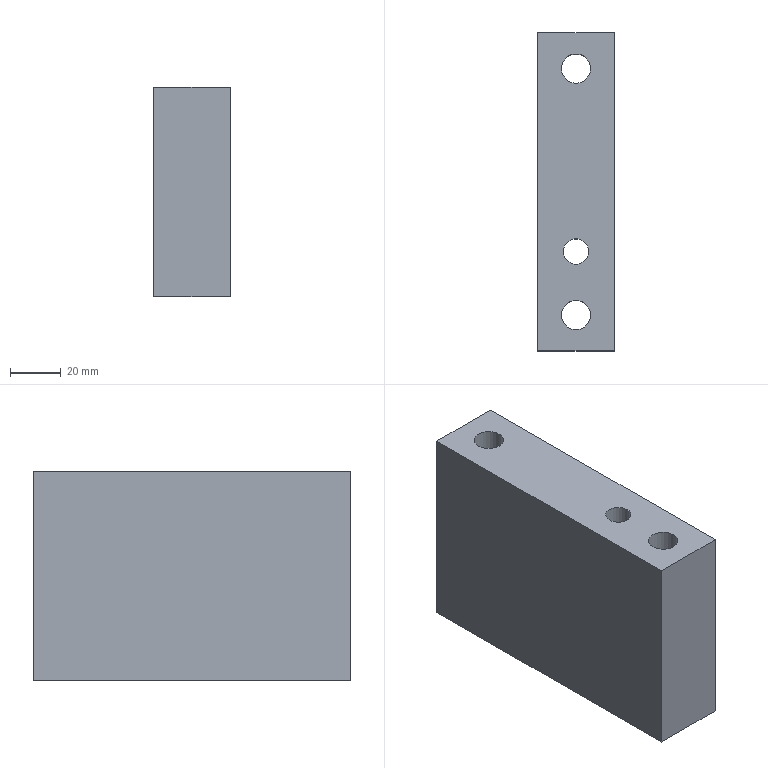Part | STEP file | lll_id3326_x_t | 1 solid | 32 faces | box 30 x 125 x 82.5 mm | volume 256192 mm3 | cylinder 20 | plane 12 | commonest cylinder face diameters 11.509 x2 18.007 x2 10 x1 13 x1 19.107 x1 19.147 x1
STEP:
#1=CARTESIAN_POINT('',(2265.,173.338,0.));
#2=VERTEX_POINT('',#1);
#3=CARTESIAN_POINT('',(2260.552,168.136,0.));
#4=VERTEX_POINT('',#3);
#5=CARTESIAN_POINT('',(2254.318,177.969,0.));
#6=DIRECTION('',(0.,0.,-1.));
#7=DIRECTION('',(-1.,0.,0.));
#8=AXIS2_PLACEMENT_3D('',#5,#6,#7);
#9=CIRCLE('',#8,11.642);
#10=EDGE_CURVE('',#2,#4,#9,.T.);
#11=ORIENTED_EDGE('',*,*,#10,.T.);
#12=CARTESIAN_POINT('',(2259.805,167.674,0.));
#13=VERTEX_POINT('',#12);
#14=CARTESIAN_POINT('',(2235.43,207.856,0.));
#15=DIRECTION('',(0.,0.,-1.));
#16=DIRECTION('',(-1.,0.,0.));
#17=AXIS2_PLACEMENT_3D('',#14,#15,#16);
#18=CIRCLE('',#17,46.998);
#19=EDGE_CURVE('',#4,#13,#18,.T.);
#20=ORIENTED_EDGE('',*,*,#19,.T.);
#21=CARTESIAN_POINT('',(2245.955,159.852,0.));
#22=VERTEX_POINT('',#21);
#23=CARTESIAN_POINT('',(2124.125,91.053,0.));
#24=DIRECTION('',(-0.8708,-0.4917,0.));
#25=VECTOR('',#24,1.);
#26=LINE('',#23,#25);
#27=EDGE_CURVE('',#13,#22,#26,.T.);
#28=ORIENTED_EDGE('',*,*,#27,.T.);
#29=CARTESIAN_POINT('',(2245.15,159.31,0.));
#30=VERTEX_POINT('',#29);
#31=CARTESIAN_POINT('',(2264.255,131.809,0.));
#32=DIRECTION('',(0.,0.,1.));
#33=DIRECTION('',(-1.,0.,0.));
#34=AXIS2_PLACEMENT_3D('',#31,#32,#33);
#35=CIRCLE('',#34,33.486);
#36=EDGE_CURVE('',#22,#30,#35,.T.);
#37=ORIENTED_EDGE('',*,*,#36,.T.);
#38=CARTESIAN_POINT('',(2244.347,158.71,0.));
#39=VERTEX_POINT('',#38);
#40=CARTESIAN_POINT('',(2252.954,148.02,0.));
#41=DIRECTION('',(0.,0.,1.));
#42=DIRECTION('',(-1.,0.,0.));
#43=AXIS2_PLACEMENT_3D('',#40,#41,#42);
#44=CIRCLE('',#43,13.725);
#45=EDGE_CURVE('',#30,#39,#44,.T.);
#46=ORIENTED_EDGE('',*,*,#45,.T.);
#47=CARTESIAN_POINT('',(2242.982,157.369,0.));
#48=VERTEX_POINT('',#47);
#49=CARTESIAN_POINT('',(2250.34,151.245,0.));
#50=DIRECTION('',(0.,0.,1.));
#51=DIRECTION('',(-1.,0.,0.));
#52=AXIS2_PLACEMENT_3D('',#49,#50,#51);
#53=CIRCLE('',#52,9.573);
#54=EDGE_CURVE('',#39,#48,#53,.T.);
#55=ORIENTED_EDGE('',*,*,#54,.T.);
#56=CARTESIAN_POINT('',(2240.441,151.267,0.));
#57=VERTEX_POINT('',#56);
#58=CARTESIAN_POINT('',(2251.719,150.151,0.));
#59=DIRECTION('',(0.,0.,1.));
#60=DIRECTION('',(-1.,0.,0.));
#61=AXIS2_PLACEMENT_3D('',#58,#59,#60);
#62=CIRCLE('',#61,11.334);
#63=EDGE_CURVE('',#48,#57,#62,.T.);
#64=ORIENTED_EDGE('',*,*,#63,.T.);
#65=CARTESIAN_POINT('',(2244.304,142.034,0.));
#66=VERTEX_POINT('',#65);
#67=CARTESIAN_POINT('',(2251.482,150.461,0.));
#68=DIRECTION('',(0.,0.,-1.));
#69=DIRECTION('',(-1.,0.,0.));
#70=AXIS2_PLACEMENT_3D('',#67,#68,#69);
#71=CIRCLE('',#70,11.07);
#72=EDGE_CURVE('',#66,#57,#71,.T.);
#73=ORIENTED_EDGE('',*,*,#72,.F.);
#74=CARTESIAN_POINT('',(2245.194,141.368,0.));
#75=VERTEX_POINT('',#74);
#76=CARTESIAN_POINT('',(2251.305,150.47,0.));
#77=DIRECTION('',(0.,0.,-1.));
#78=DIRECTION('',(-1.,0.,0.));
#79=AXIS2_PLACEMENT_3D('',#76,#77,#78);
#80=CIRCLE('',#79,10.964);
#81=EDGE_CURVE('',#75,#66,#80,.T.);
#82=ORIENTED_EDGE('',*,*,#81,.F.);
#83=CARTESIAN_POINT('',(2246.008,140.845,0.));
#84=VERTEX_POINT('',#83);
#85=CARTESIAN_POINT('',(2258.447,161.108,0.));
#86=DIRECTION('',(0.,0.,-1.));
#87=DIRECTION('',(-1.,0.,0.));
#88=AXIS2_PLACEMENT_3D('',#85,#86,#87);
#89=CIRCLE('',#88,23.776);
#90=EDGE_CURVE('',#84,#75,#89,.T.);
#91=ORIENTED_EDGE('',*,*,#90,.F.);
#92=CARTESIAN_POINT('',(2259.795,133.095,0.));
#93=VERTEX_POINT('',#92);
#94=CARTESIAN_POINT('',(2403.433,52.349,0.));
#95=DIRECTION('',(-0.8717,0.49,0.));
#96=VECTOR('',#95,1.);
#97=LINE('',#94,#96);
#98=EDGE_CURVE('',#93,#84,#97,.T.);
#99=ORIENTED_EDGE('',*,*,#98,.F.);
#100=CARTESIAN_POINT('',(2260.503,132.626,0.));
#101=VERTEX_POINT('',#100);
#102=CARTESIAN_POINT('',(2230.701,88.407,0.));
#103=DIRECTION('',(0.,0.,1.));
#104=DIRECTION('',(-1.,0.,0.));
#105=AXIS2_PLACEMENT_3D('',#102,#103,#104);
#106=CIRCLE('',#105,53.324);
#107=EDGE_CURVE('',#101,#93,#106,.T.);
#108=ORIENTED_EDGE('',*,*,#107,.F.);
#109=CARTESIAN_POINT('',(2261.24,132.116,0.));
#110=VERTEX_POINT('',#109);
#111=CARTESIAN_POINT('',(2244.874,109.242,0.));
#112=DIRECTION('',(0.,0.,1.));
#113=DIRECTION('',(-1.,0.,0.));
#114=AXIS2_PLACEMENT_3D('',#111,#112,#113);
#115=CIRCLE('',#114,28.126);
#116=EDGE_CURVE('',#110,#101,#115,.T.);
#117=ORIENTED_EDGE('',*,*,#116,.F.);
#118=CARTESIAN_POINT('',(2261.899,131.617,0.));
#119=VERTEX_POINT('',#118);
#120=CARTESIAN_POINT('',(2252.238,119.534,0.));
#121=DIRECTION('',(0.,0.,1.));
#122=DIRECTION('',(-1.,0.,0.));
#123=AXIS2_PLACEMENT_3D('',#120,#121,#122);
#124=CIRCLE('',#123,15.471);
#125=EDGE_CURVE('',#119,#110,#124,.T.);
#126=ORIENTED_EDGE('',*,*,#125,.F.);
#127=CARTESIAN_POINT('',(2262.589,131.012,0.));
#128=VERTEX_POINT('',#127);
#129=CARTESIAN_POINT('',(2255.947,124.145,0.));
#130=DIRECTION('',(0.,0.,1.));
#131=DIRECTION('',(-1.,0.,0.));
#132=AXIS2_PLACEMENT_3D('',#129,#130,#131);
#133=CIRCLE('',#132,9.553);
#134=EDGE_CURVE('',#128,#119,#133,.T.);
#135=ORIENTED_EDGE('',*,*,#134,.F.);
#136=CARTESIAN_POINT('',(2265.,127.474,0.));
#137=VERTEX_POINT('',#136);
#138=CARTESIAN_POINT('',(2254.53,122.929,0.));
#139=DIRECTION('',(0.,0.,1.));
#140=DIRECTION('',(-1.,0.,0.));
#141=AXIS2_PLACEMENT_3D('',#138,#139,#140);
#142=CIRCLE('',#141,11.414);
#143=EDGE_CURVE('',#137,#128,#142,.T.);
#144=ORIENTED_EDGE('',*,*,#143,.F.);
#145=CARTESIAN_POINT('',(2265.,75.,0.));
#146=VERTEX_POINT('',#145);
#147=CARTESIAN_POINT('',(2265.,4.,0.));
#148=DIRECTION('',(0.,1.,0.));
#149=VECTOR('',#148,1.);
#150=LINE('',#147,#149);
#151=EDGE_CURVE('',#146,#137,#150,.T.);
#152=ORIENTED_EDGE('',*,*,#151,.F.);
#153=CARTESIAN_POINT('',(2235.,75.,0.));
#154=VERTEX_POINT('',#153);
#155=CARTESIAN_POINT('',(2275.,75.,0.));
#156=DIRECTION('',(1.,0.,0.));
#157=VECTOR('',#156,1.);
#158=LINE('',#155,#157);
#159=EDGE_CURVE('',#154,#146,#158,.T.);
#160=ORIENTED_EDGE('',*,*,#159,.F.);
#161=CARTESIAN_POINT('',(2235.,200.,0.));
#162=VERTEX_POINT('',#161);
#163=CARTESIAN_POINT('',(2235.,-176.117,0.));
#164=DIRECTION('',(0.,1.,0.));
#165=VECTOR('',#164,1.);
#166=LINE('',#163,#165);
#167=EDGE_CURVE('',#154,#162,#166,.T.);
#168=ORIENTED_EDGE('',*,*,#167,.T.);
#169=CARTESIAN_POINT('',(2265.,200.,0.));
#170=VERTEX_POINT('',#169);
#171=CARTESIAN_POINT('',(2250.,200.,0.));
#172=DIRECTION('',(-1.,0.,0.));
#173=VECTOR('',#172,1.);
#174=LINE('',#171,#173);
#175=EDGE_CURVE('',#170,#162,#174,.T.);
#176=ORIENTED_EDGE('',*,*,#175,.F.);
#177=CARTESIAN_POINT('',(2265.,4.,0.));
#178=DIRECTION('',(0.,1.,0.));
#179=VECTOR('',#178,1.);
#180=LINE('',#177,#179);
#181=EDGE_CURVE('',#2,#170,#180,.T.);
#182=ORIENTED_EDGE('',*,*,#181,.F.);
#183=EDGE_LOOP('',(#11,#20,#28,#37,#46,#55,#64,#73,#82,#91,#99,#108,#117,#126,#135,#144,#152,#160,#168,#176,#182));
#184=FACE_BOUND('',#183,.T.);
#185=CARTESIAN_POINT('',(2240.997,89.,0.));
#186=VERTEX_POINT('',#185);
#187=CARTESIAN_POINT('',(2250.,89.,0.));
#188=DIRECTION('',(0.,0.,-1.));
#189=DIRECTION('',(-1.,0.,0.));
#190=AXIS2_PLACEMENT_3D('',#187,#188,#189);
#191=CIRCLE('',#190,9.004);
#192=EDGE_CURVE('',#186,#186,#191,.T.);
#193=ORIENTED_EDGE('',*,*,#192,.F.);
#194=EDGE_LOOP('',(#193));
#195=FACE_BOUND('',#194,.T.);
#196=CARTESIAN_POINT('',(2240.997,186.,0.));
#197=VERTEX_POINT('',#196);
#198=CARTESIAN_POINT('',(2250.,186.,0.));
#199=DIRECTION('',(0.,0.,-1.));
#200=DIRECTION('',(-1.,0.,0.));
#201=AXIS2_PLACEMENT_3D('',#198,#199,#200);
#202=CIRCLE('',#201,9.004);
#203=EDGE_CURVE('',#197,#197,#202,.T.);
#204=ORIENTED_EDGE('',*,*,#203,.F.);
#205=EDGE_LOOP('',(#204));
#206=FACE_BOUND('',#205,.T.);
#207=CARTESIAN_POINT('',(2256.5,114.,0.));
#208=VERTEX_POINT('',#207);
#209=CARTESIAN_POINT('',(2250.,114.,0.));
#210=DIRECTION('',(0.,0.,1.));
#211=DIRECTION('',(1.,0.,0.));
#212=AXIS2_PLACEMENT_3D('',#209,#210,#211);
#213=CIRCLE('',#212,6.5);
#214=EDGE_CURVE('',#208,#208,#213,.T.);
#215=ORIENTED_EDGE('',*,*,#214,.T.);
#216=EDGE_LOOP('',(#215));
#217=FACE_BOUND('',#216,.T.);
#218=CARTESIAN_POINT('',(2275.,-176.117,0.));
#219=DIRECTION('',(0.,0.,-1.));
#220=DIRECTION('',(-1.,0.,0.));
#221=AXIS2_PLACEMENT_3D('',#218,#219,#220);
#222=PLANE('',#221);
#223=ADVANCED_FACE('',(#184,#195,#206,#217),#222,.T.);
#224=CARTESIAN_POINT('',(2259.003,186.,52.5));
#225=VERTEX_POINT('',#224);
#226=CARTESIAN_POINT('',(2250.,186.,52.5));
#227=DIRECTION('',(0.,0.,-1.));
#228=DIRECTION('',(1.,0.,0.));
#229=AXIS2_PLACEMENT_3D('',#226,#227,#228);
#230=CIRCLE('',#229,9.004);
#231=EDGE_CURVE('',#225,#225,#230,.T.);
#232=ORIENTED_EDGE('',*,*,#231,.F.);
#233=EDGE_LOOP('',(#232));
#234=FACE_BOUND('',#233,.T.);
#235=ORIENTED_EDGE('',*,*,#203,.T.);
#236=EDGE_LOOP('',(#235));
#237=FACE_BOUND('',#236,.T.);
#238=CARTESIAN_POINT('',(2250.,186.,2.5));
#239=DIRECTION('',(0.,0.,1.));
#240=DIRECTION('',(1.,0.,0.));
#241=AXIS2_PLACEMENT_3D('',#238,#239,#240);
#242=CYLINDRICAL_SURFACE('',#241,9.004);
#243=ADVANCED_FACE('',(#234,#237),#242,.F.);
#244=CARTESIAN_POINT('',(2259.003,89.,52.5));
#245=VERTEX_POINT('',#244);
#246=CARTESIAN_POINT('',(2250.,89.,52.5));
#247=DIRECTION('',(0.,0.,-1.));
#248=DIRECTION('',(1.,0.,0.));
#249=AXIS2_PLACEMENT_3D('',#246,#247,#248);
#250=CIRCLE('',#249,9.004);
#251=EDGE_CURVE('',#245,#245,#250,.T.);
#252=ORIENTED_EDGE('',*,*,#251,.F.);
#253=EDGE_LOOP('',(#252));
#254=FACE_BOUND('',#253,.T.);
#255=ORIENTED_EDGE('',*,*,#192,.T.);
#256=EDGE_LOOP('',(#255));
#257=FACE_BOUND('',#256,.T.);
#258=CARTESIAN_POINT('',(2250.,89.,2.5));
#259=DIRECTION('',(0.,0.,1.));
#260=DIRECTION('',(1.,0.,0.));
#261=AXIS2_PLACEMENT_3D('',#258,#259,#260);
#262=CYLINDRICAL_SURFACE('',#261,9.004);
#263=ADVANCED_FACE('',(#254,#257),#262,.F.);
#264=CARTESIAN_POINT('',(2265.,127.474,17.));
#265=VERTEX_POINT('',#264);
#266=CARTESIAN_POINT('',(2265.,127.474,2.5));
#267=DIRECTION('',(0.,0.,1.));
#268=VECTOR('',#267,1.);
#269=LINE('',#266,#268);
#270=EDGE_CURVE('',#137,#265,#269,.T.);
#271=ORIENTED_EDGE('',*,*,#270,.T.);
#272=CARTESIAN_POINT('',(2265.,173.338,17.));
#273=VERTEX_POINT('',#272);
#274=CARTESIAN_POINT('',(2265.,4.,17.));
#275=DIRECTION('',(0.,1.,0.));
#276=VECTOR('',#275,1.);
#277=LINE('',#274,#276);
#278=EDGE_CURVE('',#265,#273,#277,.T.);
#279=ORIENTED_EDGE('',*,*,#278,.T.);
#280=CARTESIAN_POINT('',(2265.,173.338,5.5));
#281=DIRECTION('',(0.,0.,-1.));
#282=VECTOR('',#281,1.);
#283=LINE('',#280,#282);
#284=EDGE_CURVE('',#273,#2,#283,.T.);
#285=ORIENTED_EDGE('',*,*,#284,.T.);
#286=ORIENTED_EDGE('',*,*,#181,.T.);
#287=CARTESIAN_POINT('',(2265.,200.,82.5));
#288=VERTEX_POINT('',#287);
#289=CARTESIAN_POINT('',(2265.,200.,-652.5));
#290=DIRECTION('',(0.,0.,-1.));
#291=VECTOR('',#290,1.);
#292=LINE('',#289,#291);
#293=EDGE_CURVE('',#288,#170,#292,.T.);
#294=ORIENTED_EDGE('',*,*,#293,.F.);
#295=CARTESIAN_POINT('',(2265.,75.,82.5));
#296=VERTEX_POINT('',#295);
#297=CARTESIAN_POINT('',(2265.,4.,82.5));
#298=DIRECTION('',(0.,-1.,0.));
#299=VECTOR('',#298,1.);
#300=LINE('',#297,#299);
#301=EDGE_CURVE('',#288,#296,#300,.T.);
#302=ORIENTED_EDGE('',*,*,#301,.T.);
#303=CARTESIAN_POINT('',(2265.,75.,40.));
#304=DIRECTION('',(0.,0.,-1.));
#305=VECTOR('',#304,1.);
#306=LINE('',#303,#305);
#307=EDGE_CURVE('',#296,#146,#306,.T.);
#308=ORIENTED_EDGE('',*,*,#307,.T.);
#309=ORIENTED_EDGE('',*,*,#151,.T.);
#310=EDGE_LOOP('',(#271,#279,#285,#286,#294,#302,#308,#309));
#311=FACE_OUTER_BOUND('',#310,.T.);
#312=CARTESIAN_POINT('',(2265.,4.,-652.5));
#313=DIRECTION('',(-1.,0.,0.));
#314=DIRECTION('',(0.,0.,1.));
#315=AXIS2_PLACEMENT_3D('',#312,#313,#314);
#316=PLANE('',#315);
#317=ADVANCED_FACE('',(#311),#316,.F.);
#318=CARTESIAN_POINT('',(2255.755,186.,82.5));
#319=VERTEX_POINT('',#318);
#320=CARTESIAN_POINT('',(2250.,186.,82.5));
#321=DIRECTION('',(0.,0.,-1.));
#322=DIRECTION('',(1.,0.,0.));
#323=AXIS2_PLACEMENT_3D('',#320,#321,#322);
#324=CIRCLE('',#323,5.755);
#325=EDGE_CURVE('',#319,#319,#324,.T.);
#326=ORIENTED_EDGE('',*,*,#325,.T.);
#327=EDGE_LOOP('',(#326));
#328=FACE_BOUND('',#327,.T.);
#329=CARTESIAN_POINT('',(2255.755,89.,82.5));
#330=VERTEX_POINT('',#329);
#331=CARTESIAN_POINT('',(2250.,89.,82.5));
#332=DIRECTION('',(0.,0.,-1.));
#333=DIRECTION('',(1.,0.,0.));
#334=AXIS2_PLACEMENT_3D('',#331,#332,#333);
#335=CIRCLE('',#334,5.755);
#336=EDGE_CURVE('',#330,#330,#335,.T.);
#337=ORIENTED_EDGE('',*,*,#336,.T.);
#338=EDGE_LOOP('',(#337));
#339=FACE_BOUND('',#338,.T.);
#340=CARTESIAN_POINT('',(2255.,114.,82.5));
#341=VERTEX_POINT('',#340);
#342=CARTESIAN_POINT('',(2250.,114.,82.5));
#343=DIRECTION('',(0.,0.,-1.));
#344=DIRECTION('',(1.,0.,0.));
#345=AXIS2_PLACEMENT_3D('',#342,#343,#344);
#346=CIRCLE('',#345,5.);
#347=EDGE_CURVE('',#341,#341,#346,.T.);
#348=ORIENTED_EDGE('',*,*,#347,.T.);
#349=EDGE_LOOP('',(#348));
#350=FACE_BOUND('',#349,.T.);
#351=CARTESIAN_POINT('',(2235.,200.,82.5));
#352=VERTEX_POINT('',#351);
#353=CARTESIAN_POINT('',(2275.,200.,82.5));
#354=DIRECTION('',(-1.,0.,0.));
#355=VECTOR('',#354,1.);
#356=LINE('',#353,#355);
#357=EDGE_CURVE('',#288,#352,#356,.T.);
#358=ORIENTED_EDGE('',*,*,#357,.T.);
#359=CARTESIAN_POINT('',(2235.,75.,82.5));
#360=VERTEX_POINT('',#359);
#361=CARTESIAN_POINT('',(2235.,4.,82.5));
#362=DIRECTION('',(0.,-1.,0.));
#363=VECTOR('',#362,1.);
#364=LINE('',#361,#363);
#365=EDGE_CURVE('',#352,#360,#364,.T.);
#366=ORIENTED_EDGE('',*,*,#365,.T.);
#367=CARTESIAN_POINT('',(2275.,75.,82.5));
#368=DIRECTION('',(1.,0.,0.));
#369=VECTOR('',#368,1.);
#370=LINE('',#367,#369);
#371=EDGE_CURVE('',#360,#296,#370,.T.);
#372=ORIENTED_EDGE('',*,*,#371,.T.);
#373=ORIENTED_EDGE('',*,*,#301,.F.);
#374=EDGE_LOOP('',(#358,#366,#372,#373));
#375=FACE_BOUND('',#374,.T.);
#376=CARTESIAN_POINT('',(2275.,236.117,82.5));
#377=DIRECTION('',(0.,0.,1.));
#378=DIRECTION('',(1.,0.,0.));
#379=AXIS2_PLACEMENT_3D('',#376,#377,#378);
#380=PLANE('',#379);
#381=ADVANCED_FACE('',(#328,#339,#350,#375),#380,.T.);
#382=CARTESIAN_POINT('',(2235.,200.,40.));
#383=DIRECTION('',(0.,0.,1.));
#384=VECTOR('',#383,1.);
#385=LINE('',#382,#384);
#386=EDGE_CURVE('',#162,#352,#385,.T.);
#387=ORIENTED_EDGE('',*,*,#386,.F.);
#388=ORIENTED_EDGE('',*,*,#167,.F.);
#389=CARTESIAN_POINT('',(2235.,75.,-652.5));
#390=DIRECTION('',(0.,0.,1.));
#391=VECTOR('',#390,1.);
#392=LINE('',#389,#391);
#393=EDGE_CURVE('',#154,#360,#392,.T.);
#394=ORIENTED_EDGE('',*,*,#393,.T.);
#395=ORIENTED_EDGE('',*,*,#365,.F.);
#396=EDGE_LOOP('',(#387,#388,#394,#395));
#397=FACE_OUTER_BOUND('',#396,.T.);
#398=CARTESIAN_POINT('',(2235.,4.,-652.5));
#399=DIRECTION('',(-1.,0.,0.));
#400=DIRECTION('',(0.,0.,1.));
#401=AXIS2_PLACEMENT_3D('',#398,#399,#400);
#402=PLANE('',#401);
#403=ADVANCED_FACE('',(#397),#402,.T.);
#404=ORIENTED_EDGE('',*,*,#159,.T.);
#405=ORIENTED_EDGE('',*,*,#307,.F.);
#406=ORIENTED_EDGE('',*,*,#371,.F.);
#407=ORIENTED_EDGE('',*,*,#393,.F.);
#408=EDGE_LOOP('',(#404,#405,#406,#407));
#409=FACE_OUTER_BOUND('',#408,.T.);
#410=CARTESIAN_POINT('',(2536.,75.,40.));
#411=DIRECTION('',(0.,1.,0.));
#412=DIRECTION('',(0.,0.,-1.));
#413=AXIS2_PLACEMENT_3D('',#410,#411,#412);
#414=PLANE('',#413);
#415=ADVANCED_FACE('',(#409),#414,.F.);
#416=ORIENTED_EDGE('',*,*,#357,.F.);
#417=ORIENTED_EDGE('',*,*,#293,.T.);
#418=ORIENTED_EDGE('',*,*,#175,.T.);
#419=ORIENTED_EDGE('',*,*,#386,.T.);
#420=EDGE_LOOP('',(#416,#417,#418,#419));
#421=FACE_OUTER_BOUND('',#420,.T.);
#422=CARTESIAN_POINT('',(2250.,200.,40.));
#423=DIRECTION('',(0.,-1.,0.));
#424=DIRECTION('',(0.,0.,1.));
#425=AXIS2_PLACEMENT_3D('',#422,#423,#424);
#426=PLANE('',#425);
#427=ADVANCED_FACE('',(#421),#426,.F.);
#428=ORIENTED_EDGE('',*,*,#270,.F.);
#429=ORIENTED_EDGE('',*,*,#143,.T.);
#430=CARTESIAN_POINT('',(2262.589,131.012,17.));
#431=VERTEX_POINT('',#430);
#432=CARTESIAN_POINT('',(2262.589,131.012,5.5));
#433=DIRECTION('',(0.,0.,-1.));
#434=VECTOR('',#433,1.);
#435=LINE('',#432,#434);
#436=EDGE_CURVE('',#431,#128,#435,.T.);
#437=ORIENTED_EDGE('',*,*,#436,.F.);
#438=CARTESIAN_POINT('',(2254.53,122.929,17.));
#439=DIRECTION('',(0.,0.,-1.));
#440=DIRECTION('',(-1.,0.,0.));
#441=AXIS2_PLACEMENT_3D('',#438,#439,#440);
#442=CIRCLE('',#441,11.414);
#443=EDGE_CURVE('',#431,#265,#442,.T.);
#444=ORIENTED_EDGE('',*,*,#443,.T.);
#445=EDGE_LOOP('',(#428,#429,#437,#444));
#446=FACE_OUTER_BOUND('',#445,.T.);
#447=CARTESIAN_POINT('',(2254.53,122.929,2.5));
#448=DIRECTION('',(0.,0.,-1.));
#449=DIRECTION('',(-1.,0.,0.));
#450=AXIS2_PLACEMENT_3D('',#447,#448,#449);
#451=CYLINDRICAL_SURFACE('',#450,11.414);
#452=ADVANCED_FACE('',(#446),#451,.T.);
#453=ORIENTED_EDGE('',*,*,#284,.F.);
#454=CARTESIAN_POINT('',(2260.552,168.136,17.));
#455=VERTEX_POINT('',#454);
#456=CARTESIAN_POINT('',(2254.318,177.969,17.));
#457=DIRECTION('',(0.,0.,1.));
#458=DIRECTION('',(-1.,0.,0.));
#459=AXIS2_PLACEMENT_3D('',#456,#457,#458);
#460=CIRCLE('',#459,11.642);
#461=EDGE_CURVE('',#455,#273,#460,.T.);
#462=ORIENTED_EDGE('',*,*,#461,.F.);
#463=CARTESIAN_POINT('',(2260.552,168.136,2.5));
#464=DIRECTION('',(0.,0.,-1.));
#465=VECTOR('',#464,1.);
#466=LINE('',#463,#465);
#467=EDGE_CURVE('',#455,#4,#466,.T.);
#468=ORIENTED_EDGE('',*,*,#467,.T.);
#469=ORIENTED_EDGE('',*,*,#10,.F.);
#470=EDGE_LOOP('',(#453,#462,#468,#469));
#471=FACE_OUTER_BOUND('',#470,.T.);
#472=CARTESIAN_POINT('',(2254.318,177.969,2.5));
#473=DIRECTION('',(0.,0.,-1.));
#474=DIRECTION('',(-1.,0.,0.));
#475=AXIS2_PLACEMENT_3D('',#472,#473,#474);
#476=CYLINDRICAL_SURFACE('',#475,11.642);
#477=ADVANCED_FACE('',(#471),#476,.T.);
#478=ORIENTED_EDGE('',*,*,#278,.F.);
#479=ORIENTED_EDGE('',*,*,#443,.F.);
#480=CARTESIAN_POINT('',(2261.899,131.617,17.));
#481=VERTEX_POINT('',#480);
#482=CARTESIAN_POINT('',(2255.947,124.145,17.));
#483=DIRECTION('',(0.,0.,-1.));
#484=DIRECTION('',(-1.,0.,0.));
#485=AXIS2_PLACEMENT_3D('',#482,#483,#484);
#486=CIRCLE('',#485,9.553);
#487=EDGE_CURVE('',#481,#431,#486,.T.);
#488=ORIENTED_EDGE('',*,*,#487,.F.);
#489=CARTESIAN_POINT('',(2261.24,132.116,17.));
#490=VERTEX_POINT('',#489);
#491=CARTESIAN_POINT('',(2252.238,119.534,17.));
#492=DIRECTION('',(0.,0.,-1.));
#493=DIRECTION('',(-1.,0.,0.));
#494=AXIS2_PLACEMENT_3D('',#491,#492,#493);
#495=CIRCLE('',#494,15.471);
#496=EDGE_CURVE('',#490,#481,#495,.T.);
#497=ORIENTED_EDGE('',*,*,#496,.F.);
#498=CARTESIAN_POINT('',(2260.503,132.626,17.));
#499=VERTEX_POINT('',#498);
#500=CARTESIAN_POINT('',(2244.874,109.242,17.));
#501=DIRECTION('',(0.,0.,-1.));
#502=DIRECTION('',(-1.,0.,0.));
#503=AXIS2_PLACEMENT_3D('',#500,#501,#502);
#504=CIRCLE('',#503,28.126);
#505=EDGE_CURVE('',#499,#490,#504,.T.);
#506=ORIENTED_EDGE('',*,*,#505,.F.);
#507=CARTESIAN_POINT('',(2259.795,133.095,17.));
#508=VERTEX_POINT('',#507);
#509=CARTESIAN_POINT('',(2230.701,88.407,17.));
#510=DIRECTION('',(0.,0.,-1.));
#511=DIRECTION('',(-1.,0.,0.));
#512=AXIS2_PLACEMENT_3D('',#509,#510,#511);
#513=CIRCLE('',#512,53.324);
#514=EDGE_CURVE('',#508,#499,#513,.T.);
#515=ORIENTED_EDGE('',*,*,#514,.F.);
#516=CARTESIAN_POINT('',(2246.008,140.845,17.));
#517=VERTEX_POINT('',#516);
#518=CARTESIAN_POINT('',(2259.879,133.048,17.));
#519=DIRECTION('',(0.8717,-0.49,0.));
#520=VECTOR('',#519,1.);
#521=LINE('',#518,#520);
#522=EDGE_CURVE('',#517,#508,#521,.T.);
#523=ORIENTED_EDGE('',*,*,#522,.F.);
#524=CARTESIAN_POINT('',(2245.194,141.368,17.));
#525=VERTEX_POINT('',#524);
#526=CARTESIAN_POINT('',(2258.447,161.108,17.));
#527=DIRECTION('',(0.,0.,1.));
#528=DIRECTION('',(-1.,0.,0.));
#529=AXIS2_PLACEMENT_3D('',#526,#527,#528);
#530=CIRCLE('',#529,23.776);
#531=EDGE_CURVE('',#525,#517,#530,.T.);
#532=ORIENTED_EDGE('',*,*,#531,.F.);
#533=CARTESIAN_POINT('',(2244.304,142.034,17.));
#534=VERTEX_POINT('',#533);
#535=CARTESIAN_POINT('',(2251.305,150.47,17.));
#536=DIRECTION('',(0.,0.,1.));
#537=DIRECTION('',(-1.,0.,0.));
#538=AXIS2_PLACEMENT_3D('',#535,#536,#537);
#539=CIRCLE('',#538,10.964);
#540=EDGE_CURVE('',#534,#525,#539,.T.);
#541=ORIENTED_EDGE('',*,*,#540,.F.);
#542=CARTESIAN_POINT('',(2240.441,151.267,17.));
#543=VERTEX_POINT('',#542);
#544=CARTESIAN_POINT('',(2251.482,150.461,17.));
#545=DIRECTION('',(0.,0.,1.));
#546=DIRECTION('',(-1.,0.,0.));
#547=AXIS2_PLACEMENT_3D('',#544,#545,#546);
#548=CIRCLE('',#547,11.07);
#549=EDGE_CURVE('',#543,#534,#548,.T.);
#550=ORIENTED_EDGE('',*,*,#549,.F.);
#551=CARTESIAN_POINT('',(2242.982,157.369,17.));
#552=VERTEX_POINT('',#551);
#553=CARTESIAN_POINT('',(2251.719,150.151,17.));
#554=DIRECTION('',(0.,0.,-1.));
#555=DIRECTION('',(-1.,0.,0.));
#556=AXIS2_PLACEMENT_3D('',#553,#554,#555);
#557=CIRCLE('',#556,11.334);
#558=EDGE_CURVE('',#543,#552,#557,.T.);
#559=ORIENTED_EDGE('',*,*,#558,.T.);
#560=CARTESIAN_POINT('',(2244.347,158.71,17.));
#561=VERTEX_POINT('',#560);
#562=CARTESIAN_POINT('',(2250.34,151.245,17.));
#563=DIRECTION('',(0.,0.,-1.));
#564=DIRECTION('',(-1.,0.,0.));
#565=AXIS2_PLACEMENT_3D('',#562,#563,#564);
#566=CIRCLE('',#565,9.573);
#567=EDGE_CURVE('',#552,#561,#566,.T.);
#568=ORIENTED_EDGE('',*,*,#567,.T.);
#569=CARTESIAN_POINT('',(2245.15,159.31,17.));
#570=VERTEX_POINT('',#569);
#571=CARTESIAN_POINT('',(2252.954,148.02,17.));
#572=DIRECTION('',(0.,0.,-1.));
#573=DIRECTION('',(-1.,0.,0.));
#574=AXIS2_PLACEMENT_3D('',#571,#572,#573);
#575=CIRCLE('',#574,13.725);
#576=EDGE_CURVE('',#561,#570,#575,.T.);
#577=ORIENTED_EDGE('',*,*,#576,.T.);
#578=CARTESIAN_POINT('',(2245.955,159.852,17.));
#579=VERTEX_POINT('',#578);
#580=CARTESIAN_POINT('',(2264.255,131.809,17.));
#581=DIRECTION('',(0.,0.,-1.));
#582=DIRECTION('',(-1.,0.,0.));
#583=AXIS2_PLACEMENT_3D('',#580,#581,#582);
#584=CIRCLE('',#583,33.486);
#585=EDGE_CURVE('',#570,#579,#584,.T.);
#586=ORIENTED_EDGE('',*,*,#585,.T.);
#587=CARTESIAN_POINT('',(2259.805,167.674,17.));
#588=VERTEX_POINT('',#587);
#589=CARTESIAN_POINT('',(2259.845,167.696,17.));
#590=DIRECTION('',(0.8708,0.4917,0.));
#591=VECTOR('',#590,1.);
#592=LINE('',#589,#591);
#593=EDGE_CURVE('',#579,#588,#592,.T.);
#594=ORIENTED_EDGE('',*,*,#593,.T.);
#595=CARTESIAN_POINT('',(2235.43,207.856,17.));
#596=DIRECTION('',(0.,0.,1.));
#597=DIRECTION('',(-1.,0.,0.));
#598=AXIS2_PLACEMENT_3D('',#595,#596,#597);
#599=CIRCLE('',#598,46.998);
#600=EDGE_CURVE('',#588,#455,#599,.T.);
#601=ORIENTED_EDGE('',*,*,#600,.T.);
#602=ORIENTED_EDGE('',*,*,#461,.T.);
#603=EDGE_LOOP('',(#478,#479,#488,#497,#506,#515,#523,#532,#541,#550,#559,#568,#577,#586,#594,#601,#602));
#604=FACE_OUTER_BOUND('',#603,.T.);
#605=CARTESIAN_POINT('',(13164.883,13712.786,17.));
#606=DIRECTION('',(0.,0.,-1.));
#607=DIRECTION('',(-1.,0.,0.));
#608=AXIS2_PLACEMENT_3D('',#605,#606,#607);
#609=PLANE('',#608);
#610=ADVANCED_FACE('',(#604),#609,.T.);
#611=ORIENTED_EDGE('',*,*,#134,.T.);
#612=CARTESIAN_POINT('',(2261.899,131.617,5.5));
#613=DIRECTION('',(0.,0.,-1.));
#614=VECTOR('',#613,1.);
#615=LINE('',#612,#614);
#616=EDGE_CURVE('',#481,#119,#615,.T.);
#617=ORIENTED_EDGE('',*,*,#616,.F.);
#618=ORIENTED_EDGE('',*,*,#487,.T.);
#619=ORIENTED_EDGE('',*,*,#436,.T.);
#620=EDGE_LOOP('',(#611,#617,#618,#619));
#621=FACE_OUTER_BOUND('',#620,.T.);
#622=CARTESIAN_POINT('',(2255.947,124.145,2.5));
#623=DIRECTION('',(0.,0.,-1.));
#624=DIRECTION('',(-1.,0.,0.));
#625=AXIS2_PLACEMENT_3D('',#622,#623,#624);
#626=CYLINDRICAL_SURFACE('',#625,9.553);
#627=ADVANCED_FACE('',(#621),#626,.T.);
#628=ORIENTED_EDGE('',*,*,#125,.T.);
#629=CARTESIAN_POINT('',(2261.24,132.116,2.5));
#630=DIRECTION('',(0.,0.,-1.));
#631=VECTOR('',#630,1.);
#632=LINE('',#629,#631);
#633=EDGE_CURVE('',#490,#110,#632,.T.);
#634=ORIENTED_EDGE('',*,*,#633,.F.);
#635=ORIENTED_EDGE('',*,*,#496,.T.);
#636=ORIENTED_EDGE('',*,*,#616,.T.);
#637=EDGE_LOOP('',(#628,#634,#635,#636));
#638=FACE_OUTER_BOUND('',#637,.T.);
#639=CARTESIAN_POINT('',(2252.238,119.534,2.5));
#640=DIRECTION('',(0.,0.,-1.));
#641=DIRECTION('',(-1.,0.,0.));
#642=AXIS2_PLACEMENT_3D('',#639,#640,#641);
#643=CYLINDRICAL_SURFACE('',#642,15.471);
#644=ADVANCED_FACE('',(#638),#643,.T.);
#645=ORIENTED_EDGE('',*,*,#116,.T.);
#646=CARTESIAN_POINT('',(2260.503,132.626,5.5));
#647=DIRECTION('',(0.,0.,-1.));
#648=VECTOR('',#647,1.);
#649=LINE('',#646,#648);
#650=EDGE_CURVE('',#499,#101,#649,.T.);
#651=ORIENTED_EDGE('',*,*,#650,.F.);
#652=ORIENTED_EDGE('',*,*,#505,.T.);
#653=ORIENTED_EDGE('',*,*,#633,.T.);
#654=EDGE_LOOP('',(#645,#651,#652,#653));
#655=FACE_OUTER_BOUND('',#654,.T.);
#656=CARTESIAN_POINT('',(2244.874,109.242,2.5));
#657=DIRECTION('',(0.,0.,-1.));
#658=DIRECTION('',(-1.,0.,0.));
#659=AXIS2_PLACEMENT_3D('',#656,#657,#658);
#660=CYLINDRICAL_SURFACE('',#659,28.126);
#661=ADVANCED_FACE('',(#655),#660,.T.);
#662=ORIENTED_EDGE('',*,*,#107,.T.);
#663=CARTESIAN_POINT('',(2259.795,133.095,5.5));
#664=DIRECTION('',(0.,0.,-1.));
#665=VECTOR('',#664,1.);
#666=LINE('',#663,#665);
#667=EDGE_CURVE('',#508,#93,#666,.T.);
#668=ORIENTED_EDGE('',*,*,#667,.F.);
#669=ORIENTED_EDGE('',*,*,#514,.T.);
#670=ORIENTED_EDGE('',*,*,#650,.T.);
#671=EDGE_LOOP('',(#662,#668,#669,#670));
#672=FACE_OUTER_BOUND('',#671,.T.);
#673=CARTESIAN_POINT('',(2230.701,88.407,2.5));
#674=DIRECTION('',(0.,0.,-1.));
#675=DIRECTION('',(-1.,0.,0.));
#676=AXIS2_PLACEMENT_3D('',#673,#674,#675);
#677=CYLINDRICAL_SURFACE('',#676,53.324);
#678=ADVANCED_FACE('',(#672),#677,.T.);
#679=ORIENTED_EDGE('',*,*,#98,.T.);
#680=CARTESIAN_POINT('',(2246.008,140.845,5.5));
#681=DIRECTION('',(0.,0.,-1.));
#682=VECTOR('',#681,1.);
#683=LINE('',#680,#682);
#684=EDGE_CURVE('',#517,#84,#683,.T.);
#685=ORIENTED_EDGE('',*,*,#684,.F.);
#686=ORIENTED_EDGE('',*,*,#522,.T.);
#687=ORIENTED_EDGE('',*,*,#667,.T.);
#688=EDGE_LOOP('',(#679,#685,#686,#687));
#689=FACE_OUTER_BOUND('',#688,.T.);
#690=CARTESIAN_POINT('',(2259.879,133.048,2.5));
#691=DIRECTION('',(0.49,0.8717,0.));
#692=DIRECTION('',(-0.8717,0.49,0.));
#693=AXIS2_PLACEMENT_3D('',#690,#691,#692);
#694=PLANE('',#693);
#695=ADVANCED_FACE('',(#689),#694,.T.);
#696=ORIENTED_EDGE('',*,*,#90,.T.);
#697=CARTESIAN_POINT('',(2245.194,141.368,2.5));
#698=DIRECTION('',(0.,0.,-1.));
#699=VECTOR('',#698,1.);
#700=LINE('',#697,#699);
#701=EDGE_CURVE('',#525,#75,#700,.T.);
#702=ORIENTED_EDGE('',*,*,#701,.F.);
#703=ORIENTED_EDGE('',*,*,#531,.T.);
#704=ORIENTED_EDGE('',*,*,#684,.T.);
#705=EDGE_LOOP('',(#696,#702,#703,#704));
#706=FACE_OUTER_BOUND('',#705,.T.);
#707=CARTESIAN_POINT('',(2258.447,161.108,2.5));
#708=DIRECTION('',(0.,0.,-1.));
#709=DIRECTION('',(-1.,0.,0.));
#710=AXIS2_PLACEMENT_3D('',#707,#708,#709);
#711=CYLINDRICAL_SURFACE('',#710,23.776);
#712=ADVANCED_FACE('',(#706),#711,.F.);
#713=ORIENTED_EDGE('',*,*,#81,.T.);
#714=CARTESIAN_POINT('',(2244.304,142.034,5.5));
#715=DIRECTION('',(0.,0.,-1.));
#716=VECTOR('',#715,1.);
#717=LINE('',#714,#716);
#718=EDGE_CURVE('',#534,#66,#717,.T.);
#719=ORIENTED_EDGE('',*,*,#718,.F.);
#720=ORIENTED_EDGE('',*,*,#540,.T.);
#721=ORIENTED_EDGE('',*,*,#701,.T.);
#722=EDGE_LOOP('',(#713,#719,#720,#721));
#723=FACE_OUTER_BOUND('',#722,.T.);
#724=CARTESIAN_POINT('',(2251.305,150.47,2.5));
#725=DIRECTION('',(0.,0.,-1.));
#726=DIRECTION('',(-1.,0.,0.));
#727=AXIS2_PLACEMENT_3D('',#724,#725,#726);
#728=CYLINDRICAL_SURFACE('',#727,10.964);
#729=ADVANCED_FACE('',(#723),#728,.F.);
#730=ORIENTED_EDGE('',*,*,#72,.T.);
#731=CARTESIAN_POINT('',(2240.441,151.267,5.5));
#732=DIRECTION('',(0.,0.,-1.));
#733=VECTOR('',#732,1.);
#734=LINE('',#731,#733);
#735=EDGE_CURVE('',#543,#57,#734,.T.);
#736=ORIENTED_EDGE('',*,*,#735,.F.);
#737=ORIENTED_EDGE('',*,*,#549,.T.);
#738=ORIENTED_EDGE('',*,*,#718,.T.);
#739=EDGE_LOOP('',(#730,#736,#737,#738));
#740=FACE_OUTER_BOUND('',#739,.T.);
#741=CARTESIAN_POINT('',(2251.482,150.461,2.5));
#742=DIRECTION('',(0.,0.,-1.));
#743=DIRECTION('',(-1.,0.,0.));
#744=AXIS2_PLACEMENT_3D('',#741,#742,#743);
#745=CYLINDRICAL_SURFACE('',#744,11.07);
#746=ADVANCED_FACE('',(#740),#745,.F.);
#747=ORIENTED_EDGE('',*,*,#63,.F.);
#748=CARTESIAN_POINT('',(2242.982,157.369,5.5));
#749=DIRECTION('',(0.,0.,-1.));
#750=VECTOR('',#749,1.);
#751=LINE('',#748,#750);
#752=EDGE_CURVE('',#552,#48,#751,.T.);
#753=ORIENTED_EDGE('',*,*,#752,.F.);
#754=ORIENTED_EDGE('',*,*,#558,.F.);
#755=ORIENTED_EDGE('',*,*,#735,.T.);
#756=EDGE_LOOP('',(#747,#753,#754,#755));
#757=FACE_OUTER_BOUND('',#756,.T.);
#758=CARTESIAN_POINT('',(2251.719,150.151,2.5));
#759=DIRECTION('',(0.,0.,-1.));
#760=DIRECTION('',(-1.,0.,0.));
#761=AXIS2_PLACEMENT_3D('',#758,#759,#760);
#762=CYLINDRICAL_SURFACE('',#761,11.334);
#763=ADVANCED_FACE('',(#757),#762,.F.);
#764=ORIENTED_EDGE('',*,*,#54,.F.);
#765=CARTESIAN_POINT('',(2244.347,158.71,5.5));
#766=DIRECTION('',(0.,0.,-1.));
#767=VECTOR('',#766,1.);
#768=LINE('',#765,#767);
#769=EDGE_CURVE('',#561,#39,#768,.T.);
#770=ORIENTED_EDGE('',*,*,#769,.F.);
#771=ORIENTED_EDGE('',*,*,#567,.F.);
#772=ORIENTED_EDGE('',*,*,#752,.T.);
#773=EDGE_LOOP('',(#764,#770,#771,#772));
#774=FACE_OUTER_BOUND('',#773,.T.);
#775=CARTESIAN_POINT('',(2250.34,151.245,2.5));
#776=DIRECTION('',(0.,0.,-1.));
#777=DIRECTION('',(-1.,0.,0.));
#778=AXIS2_PLACEMENT_3D('',#775,#776,#777);
#779=CYLINDRICAL_SURFACE('',#778,9.573);
#780=ADVANCED_FACE('',(#774),#779,.F.);
#781=ORIENTED_EDGE('',*,*,#45,.F.);
#782=CARTESIAN_POINT('',(2245.15,159.31,5.5));
#783=DIRECTION('',(0.,0.,-1.));
#784=VECTOR('',#783,1.);
#785=LINE('',#782,#784);
#786=EDGE_CURVE('',#570,#30,#785,.T.);
#787=ORIENTED_EDGE('',*,*,#786,.F.);
#788=ORIENTED_EDGE('',*,*,#576,.F.);
#789=ORIENTED_EDGE('',*,*,#769,.T.);
#790=EDGE_LOOP('',(#781,#787,#788,#789));
#791=FACE_OUTER_BOUND('',#790,.T.);
#792=CARTESIAN_POINT('',(2252.954,148.02,2.5));
#793=DIRECTION('',(0.,0.,-1.));
#794=DIRECTION('',(-1.,0.,0.));
#795=AXIS2_PLACEMENT_3D('',#792,#793,#794);
#796=CYLINDRICAL_SURFACE('',#795,13.725);
#797=ADVANCED_FACE('',(#791),#796,.F.);
#798=ORIENTED_EDGE('',*,*,#36,.F.);
#799=CARTESIAN_POINT('',(2245.955,159.852,5.5));
#800=DIRECTION('',(0.,0.,-1.));
#801=VECTOR('',#800,1.);
#802=LINE('',#799,#801);
#803=EDGE_CURVE('',#579,#22,#802,.T.);
#804=ORIENTED_EDGE('',*,*,#803,.F.);
#805=ORIENTED_EDGE('',*,*,#585,.F.);
#806=ORIENTED_EDGE('',*,*,#786,.T.);
#807=EDGE_LOOP('',(#798,#804,#805,#806));
#808=FACE_OUTER_BOUND('',#807,.T.);
#809=CARTESIAN_POINT('',(2264.255,131.809,2.5));
#810=DIRECTION('',(0.,0.,-1.));
#811=DIRECTION('',(-1.,0.,0.));
#812=AXIS2_PLACEMENT_3D('',#809,#810,#811);
#813=CYLINDRICAL_SURFACE('',#812,33.486);
#814=ADVANCED_FACE('',(#808),#813,.F.);
#815=ORIENTED_EDGE('',*,*,#27,.F.);
#816=CARTESIAN_POINT('',(2259.805,167.674,5.5));
#817=DIRECTION('',(0.,0.,-1.));
#818=VECTOR('',#817,1.);
#819=LINE('',#816,#818);
#820=EDGE_CURVE('',#588,#13,#819,.T.);
#821=ORIENTED_EDGE('',*,*,#820,.F.);
#822=ORIENTED_EDGE('',*,*,#593,.F.);
#823=ORIENTED_EDGE('',*,*,#803,.T.);
#824=EDGE_LOOP('',(#815,#821,#822,#823));
#825=FACE_OUTER_BOUND('',#824,.T.);
#826=CARTESIAN_POINT('',(2259.845,167.696,2.5));
#827=DIRECTION('',(-0.4917,0.8708,0.));
#828=DIRECTION('',(-0.8708,-0.4917,0.));
#829=AXIS2_PLACEMENT_3D('',#826,#827,#828);
#830=PLANE('',#829);
#831=ADVANCED_FACE('',(#825),#830,.F.);
#832=ORIENTED_EDGE('',*,*,#19,.F.);
#833=ORIENTED_EDGE('',*,*,#467,.F.);
#834=ORIENTED_EDGE('',*,*,#600,.F.);
#835=ORIENTED_EDGE('',*,*,#820,.T.);
#836=EDGE_LOOP('',(#832,#833,#834,#835));
#837=FACE_OUTER_BOUND('',#836,.T.);
#838=CARTESIAN_POINT('',(2235.43,207.856,2.5));
#839=DIRECTION('',(0.,0.,-1.));
#840=DIRECTION('',(-1.,0.,0.));
#841=AXIS2_PLACEMENT_3D('',#838,#839,#840);
#842=CYLINDRICAL_SURFACE('',#841,46.998);
#843=ADVANCED_FACE('',(#837),#842,.T.);
#844=CARTESIAN_POINT('',(2255.,114.,50.));
#845=VERTEX_POINT('',#844);
#846=CARTESIAN_POINT('',(2250.,114.,50.));
#847=DIRECTION('',(0.,0.,-1.));
#848=DIRECTION('',(1.,0.,0.));
#849=AXIS2_PLACEMENT_3D('',#846,#847,#848);
#850=CIRCLE('',#849,5.);
#851=EDGE_CURVE('',#845,#845,#850,.T.);
#852=ORIENTED_EDGE('',*,*,#851,.T.);
#853=EDGE_LOOP('',(#852));
#854=FACE_BOUND('',#853,.T.);
#855=ORIENTED_EDGE('',*,*,#347,.F.);
#856=EDGE_LOOP('',(#855));
#857=FACE_BOUND('',#856,.T.);
#858=CARTESIAN_POINT('',(2250.,114.,-2.5));
#859=DIRECTION('',(0.,0.,1.));
#860=DIRECTION('',(1.,0.,0.));
#861=AXIS2_PLACEMENT_3D('',#858,#859,#860);
#862=CYLINDRICAL_SURFACE('',#861,5.);
#863=ADVANCED_FACE('',(#854,#857),#862,.F.);
#864=ORIENTED_EDGE('',*,*,#336,.F.);
#865=EDGE_LOOP('',(#864));
#866=FACE_BOUND('',#865,.T.);
#867=CARTESIAN_POINT('',(2255.755,89.,52.5));
#868=VERTEX_POINT('',#867);
#869=CARTESIAN_POINT('',(2250.,89.,52.5));
#870=DIRECTION('',(0.,0.,-1.));
#871=DIRECTION('',(1.,0.,0.));
#872=AXIS2_PLACEMENT_3D('',#869,#870,#871);
#873=CIRCLE('',#872,5.755);
#874=EDGE_CURVE('',#868,#868,#873,.T.);
#875=ORIENTED_EDGE('',*,*,#874,.T.);
#876=EDGE_LOOP('',(#875));
#877=FACE_BOUND('',#876,.T.);
#878=CARTESIAN_POINT('',(2250.,89.,-2.5));
#879=DIRECTION('',(0.,0.,1.));
#880=DIRECTION('',(1.,0.,0.));
#881=AXIS2_PLACEMENT_3D('',#878,#879,#880);
#882=CYLINDRICAL_SURFACE('',#881,5.755);
#883=ADVANCED_FACE('',(#866,#877),#882,.F.);
#884=ORIENTED_EDGE('',*,*,#874,.F.);
#885=EDGE_LOOP('',(#884));
#886=FACE_BOUND('',#885,.T.);
#887=ORIENTED_EDGE('',*,*,#251,.T.);
#888=EDGE_LOOP('',(#887));
#889=FACE_BOUND('',#888,.T.);
#890=CARTESIAN_POINT('',(2250.,89.,52.5));
#891=DIRECTION('',(0.,0.,1.));
#892=DIRECTION('',(1.,0.,0.));
#893=AXIS2_PLACEMENT_3D('',#890,#891,#892);
#894=PLANE('',#893);
#895=ADVANCED_FACE('',(#886,#889),#894,.F.);
#896=ORIENTED_EDGE('',*,*,#325,.F.);
#897=EDGE_LOOP('',(#896));
#898=FACE_BOUND('',#897,.T.);
#899=CARTESIAN_POINT('',(2255.755,186.,52.5));
#900=VERTEX_POINT('',#899);
#901=CARTESIAN_POINT('',(2250.,186.,52.5));
#902=DIRECTION('',(0.,0.,-1.));
#903=DIRECTION('',(1.,0.,0.));
#904=AXIS2_PLACEMENT_3D('',#901,#902,#903);
#905=CIRCLE('',#904,5.755);
#906=EDGE_CURVE('',#900,#900,#905,.T.);
#907=ORIENTED_EDGE('',*,*,#906,.T.);
#908=EDGE_LOOP('',(#907));
#909=FACE_BOUND('',#908,.T.);
#910=CARTESIAN_POINT('',(2250.,186.,-2.5));
#911=DIRECTION('',(0.,0.,1.));
#912=DIRECTION('',(1.,0.,0.));
#913=AXIS2_PLACEMENT_3D('',#910,#911,#912);
#914=CYLINDRICAL_SURFACE('',#913,5.755);
#915=ADVANCED_FACE('',(#898,#909),#914,.F.);
#916=ORIENTED_EDGE('',*,*,#906,.F.);
#917=EDGE_LOOP('',(#916));
#918=FACE_BOUND('',#917,.T.);
#919=ORIENTED_EDGE('',*,*,#231,.T.);
#920=EDGE_LOOP('',(#919));
#921=FACE_BOUND('',#920,.T.);
#922=CARTESIAN_POINT('',(2250.,186.,52.5));
#923=DIRECTION('',(0.,0.,1.));
#924=DIRECTION('',(1.,0.,0.));
#925=AXIS2_PLACEMENT_3D('',#922,#923,#924);
#926=PLANE('',#925);
#927=ADVANCED_FACE('',(#918,#921),#926,.F.);
#928=CARTESIAN_POINT('',(2256.5,114.,50.));
#929=VERTEX_POINT('',#928);
#930=CARTESIAN_POINT('',(2250.,114.,50.));
#931=DIRECTION('',(0.,0.,1.));
#932=DIRECTION('',(1.,0.,0.));
#933=AXIS2_PLACEMENT_3D('',#930,#931,#932);
#934=CIRCLE('',#933,6.5);
#935=EDGE_CURVE('',#929,#929,#934,.T.);
#936=ORIENTED_EDGE('',*,*,#935,.F.);
#937=EDGE_LOOP('',(#936));
#938=FACE_BOUND('',#937,.T.);
#939=ORIENTED_EDGE('',*,*,#851,.F.);
#940=EDGE_LOOP('',(#939));
#941=FACE_BOUND('',#940,.T.);
#942=CARTESIAN_POINT('',(2250.,114.,50.));
#943=DIRECTION('',(0.,0.,1.));
#944=DIRECTION('',(1.,0.,0.));
#945=AXIS2_PLACEMENT_3D('',#942,#943,#944);
#946=PLANE('',#945);
#947=ADVANCED_FACE('',(#938,#941),#946,.F.);
#948=ORIENTED_EDGE('',*,*,#935,.T.);
#949=EDGE_LOOP('',(#948));
#950=FACE_BOUND('',#949,.T.);
#951=ORIENTED_EDGE('',*,*,#214,.F.);
#952=EDGE_LOOP('',(#951));
#953=FACE_BOUND('',#952,.T.);
#954=CARTESIAN_POINT('',(2250.,114.,0.));
#955=DIRECTION('',(0.,0.,1.));
#956=DIRECTION('',(1.,0.,0.));
#957=AXIS2_PLACEMENT_3D('',#954,#955,#956);
#958=CYLINDRICAL_SURFACE('',#957,6.5);
#959=ADVANCED_FACE('',(#950,#953),#958,.F.);
#960=CLOSED_SHELL('',(#223,#243,#263,#317,#381,#403,#415,#427,#452,#477,#610,#627,#644,#661,#678,#695,#712,#729,#746,#763,#780,#797,#814,#831,#843,#863,#883,#895,#915,#927,#947,#959));
#961=MANIFOLD_SOLID_BREP('',#960);
#962=(LENGTH_UNIT()NAMED_UNIT(*)SI_UNIT(.MILLI.,.METRE.));
#963=UNCERTAINTY_MEASURE_WITH_UNIT(LENGTH_MEASURE(0.00002),#962,'','');
#964=(NAMED_UNIT(*)PLANE_ANGLE_UNIT()SI_UNIT($,.RADIAN.));
#965=PLANE_ANGLE_MEASURE_WITH_UNIT(PLANE_ANGLE_MEASURE(0.01745),#964);
#966=DIMENSIONAL_EXPONENTS(0.,0.,0.,0.,0.,0.,0.);
#967=(CONVERSION_BASED_UNIT('DEGREE',#965)NAMED_UNIT(#966)PLANE_ANGLE_UNIT());
#968=(NAMED_UNIT(*)SI_UNIT($,.STERADIAN.)SOLID_ANGLE_UNIT());
#969=(GEOMETRIC_REPRESENTATION_CONTEXT(3)GLOBAL_UNCERTAINTY_ASSIGNED_CONTEXT((#963))GLOBAL_UNIT_ASSIGNED_CONTEXT((#962,#967,#968))REPRESENTATION_CONTEXT('',''));
#970=ADVANCED_BREP_SHAPE_REPRESENTATION('',(#961),#969);